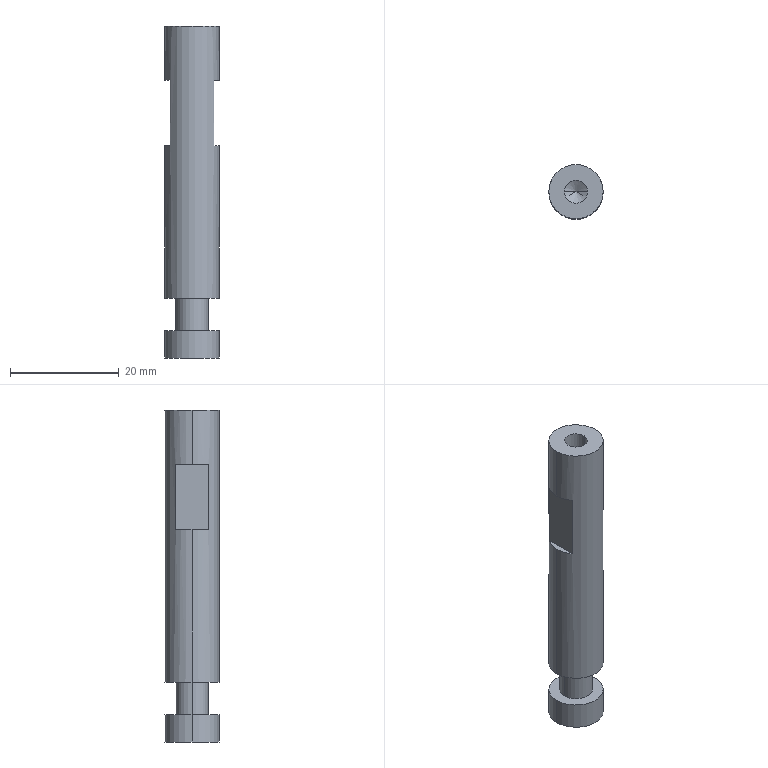Part | STEP file | 2101 Cylinder joint B | 1 solid | 20 faces | box 10 x 10 x 61 mm | volume 4191 mm3 | plane 10 | cylinder 8 | cone 2 | commonest cylinder face diameters 10 x4 4.2 x2 6 x2
STEP:
#1=CARTESIAN_POINT('',(0.,0.,0.));
#2=DIRECTION('',(0.,0.,1.));
#3=DIRECTION('',(1.,0.,0.));
#4=AXIS2_PLACEMENT_3D('',#1,#2,#3);
#5=CARTESIAN_POINT('',(2.1,0.,47.));
#6=VERTEX_POINT('',#5);
#7=CARTESIAN_POINT('',(2.1,0.,61.));
#8=VERTEX_POINT('',#7);
#9=CARTESIAN_POINT('',(2.1,0.,61.));
#10=DIRECTION('',(0.,0.,1.));
#11=VECTOR('',#10,1.);
#12=LINE('',#9,#11);
#13=CARTESIAN_POINT('',(0.,0.,61.));
#14=DIRECTION('',(0.,0.,1.));
#15=DIRECTION('',(1.,0.,0.));
#16=AXIS2_PLACEMENT_3D('',#13,#14,#15);
#17=CYLINDRICAL_SURFACE('',#16,2.1);
#18=CARTESIAN_POINT('',(6.283,0.));
#19=DIRECTION('',(0.,1.));
#20=VECTOR('',#19,1.);
#21=LINE('',#18,#20);
#22=(GEOMETRIC_REPRESENTATION_CONTEXT(2)PARAMETRIC_REPRESENTATION_CONTEXT()REPRESENTATION_CONTEXT('',''));
#23=DEFINITIONAL_REPRESENTATION('',(#21),#22);
#24=PCURVE('',#17,#23);
#25=CARTESIAN_POINT('',(0.,0.,61.));
#26=DIRECTION('',(0.,0.,1.));
#27=DIRECTION('',(1.,0.,0.));
#28=AXIS2_PLACEMENT_3D('',#25,#26,#27);
#29=CYLINDRICAL_SURFACE('',#28,2.1);
#30=CARTESIAN_POINT('',(0.,0.));
#31=DIRECTION('',(0.,1.));
#32=VECTOR('',#31,1.);
#33=LINE('',#30,#32);
#34=(GEOMETRIC_REPRESENTATION_CONTEXT(2)PARAMETRIC_REPRESENTATION_CONTEXT()REPRESENTATION_CONTEXT('',''));
#35=DEFINITIONAL_REPRESENTATION('',(#33),#34);
#36=PCURVE('',#29,#35);
#37=SURFACE_CURVE('',#12,(#24,#36),.PCURVE_S1.);
#38=EDGE_CURVE('',#6,#8,#37,.T.);
#39=ORIENTED_EDGE('',*,*,#38,.T.);
#40=CARTESIAN_POINT('',(-2.1,0.,61.));
#41=VERTEX_POINT('',#40);
#42=CARTESIAN_POINT('',(0.,0.,61.));
#43=DIRECTION('',(0.,0.,1.));
#44=DIRECTION('',(1.,0.,0.));
#45=AXIS2_PLACEMENT_3D('',#42,#43,#44);
#46=CIRCLE('',#45,2.1);
#47=CARTESIAN_POINT('',(0.,0.));
#48=DIRECTION('',(1.,0.));
#49=VECTOR('',#48,1.);
#50=LINE('',#47,#49);
#51=(GEOMETRIC_REPRESENTATION_CONTEXT(2)PARAMETRIC_REPRESENTATION_CONTEXT()REPRESENTATION_CONTEXT('',''));
#52=DEFINITIONAL_REPRESENTATION('',(#50),#51);
#53=PCURVE('',#17,#52);
#54=CARTESIAN_POINT('',(0.,0.,61.));
#55=DIRECTION('',(0.,0.,1.));
#56=DIRECTION('',(1.,0.,0.));
#57=AXIS2_PLACEMENT_3D('',#54,#55,#56);
#58=PLANE('',#57);
#59=CARTESIAN_POINT('',(0.,0.));
#60=DIRECTION('',(1.,0.));
#61=AXIS2_PLACEMENT_2D('',#59,#60);
#62=CIRCLE('',#61,2.1);
#63=(GEOMETRIC_REPRESENTATION_CONTEXT(2)PARAMETRIC_REPRESENTATION_CONTEXT()REPRESENTATION_CONTEXT('',''));
#64=DEFINITIONAL_REPRESENTATION('',(#62),#63);
#65=PCURVE('',#58,#64);
#66=SURFACE_CURVE('',#46,(#53,#65),.PCURVE_S1.);
#67=EDGE_CURVE('',#41,#8,#66,.T.);
#68=ORIENTED_EDGE('',*,*,#67,.F.);
#69=CARTESIAN_POINT('',(-2.1,0.,47.));
#70=VERTEX_POINT('',#69);
#71=CARTESIAN_POINT('',(-2.1,0.,61.));
#72=DIRECTION('',(0.,0.,1.));
#73=VECTOR('',#72,1.);
#74=LINE('',#71,#73);
#75=CARTESIAN_POINT('',(3.142,0.));
#76=DIRECTION('',(0.,1.));
#77=VECTOR('',#76,1.);
#78=LINE('',#75,#77);
#79=(GEOMETRIC_REPRESENTATION_CONTEXT(2)PARAMETRIC_REPRESENTATION_CONTEXT()REPRESENTATION_CONTEXT('',''));
#80=DEFINITIONAL_REPRESENTATION('',(#78),#79);
#81=PCURVE('',#17,#80);
#82=CARTESIAN_POINT('',(3.142,0.));
#83=DIRECTION('',(0.,1.));
#84=VECTOR('',#83,1.);
#85=LINE('',#82,#84);
#86=(GEOMETRIC_REPRESENTATION_CONTEXT(2)PARAMETRIC_REPRESENTATION_CONTEXT()REPRESENTATION_CONTEXT('',''));
#87=DEFINITIONAL_REPRESENTATION('',(#85),#86);
#88=PCURVE('',#29,#87);
#89=SURFACE_CURVE('',#74,(#81,#88),.PCURVE_S1.);
#90=EDGE_CURVE('',#70,#41,#89,.T.);
#91=ORIENTED_EDGE('',*,*,#90,.F.);
#92=CARTESIAN_POINT('',(0.,0.,47.));
#93=DIRECTION('',(0.,0.,1.));
#94=DIRECTION('',(1.,0.,0.));
#95=AXIS2_PLACEMENT_3D('',#92,#93,#94);
#96=CIRCLE('',#95,2.1);
#97=CARTESIAN_POINT('',(0.,-14.));
#98=DIRECTION('',(1.,0.));
#99=VECTOR('',#98,1.);
#100=LINE('',#97,#99);
#101=(GEOMETRIC_REPRESENTATION_CONTEXT(2)PARAMETRIC_REPRESENTATION_CONTEXT()REPRESENTATION_CONTEXT('',''));
#102=DEFINITIONAL_REPRESENTATION('',(#100),#101);
#103=PCURVE('',#17,#102);
#104=CARTESIAN_POINT('',(0.,0.,47.));
#105=DIRECTION('',(0.,0.,1.));
#106=DIRECTION('',(1.,0.,0.));
#107=AXIS2_PLACEMENT_3D('',#104,#105,#106);
#108=CONICAL_SURFACE('',#107,2.1,1.03);
#109=CARTESIAN_POINT('',(0.,0.));
#110=DIRECTION('',(1.,0.));
#111=VECTOR('',#110,1.);
#112=LINE('',#109,#111);
#113=(GEOMETRIC_REPRESENTATION_CONTEXT(2)PARAMETRIC_REPRESENTATION_CONTEXT()REPRESENTATION_CONTEXT('',''));
#114=DEFINITIONAL_REPRESENTATION('',(#112),#113);
#115=PCURVE('',#108,#114);
#116=SURFACE_CURVE('',#96,(#103,#115),.PCURVE_S1.);
#117=EDGE_CURVE('',#70,#6,#116,.T.);
#118=ORIENTED_EDGE('',*,*,#117,.T.);
#119=EDGE_LOOP('',(#39,#68,#91,#118));
#120=FACE_BOUND('',#119,.F.);
#121=ADVANCED_FACE('',(#120),#17,.F.);
#122=ORIENTED_EDGE('',*,*,#117,.F.);
#123=CARTESIAN_POINT('',(0.,0.,45.738));
#124=VERTEX_POINT('',#123);
#125=CARTESIAN_POINT('',(-2.1,0.,47.));
#126=DIRECTION('',(-0.8572,0.,0.515));
#127=VECTOR('',#126,1.);
#128=LINE('',#125,#127);
#129=CARTESIAN_POINT('',(3.142,0.));
#130=DIRECTION('',(0.,1.));
#131=VECTOR('',#130,1.);
#132=LINE('',#129,#131);
#133=(GEOMETRIC_REPRESENTATION_CONTEXT(2)PARAMETRIC_REPRESENTATION_CONTEXT()REPRESENTATION_CONTEXT('',''));
#134=DEFINITIONAL_REPRESENTATION('',(#132),#133);
#135=PCURVE('',#108,#134);
#136=CARTESIAN_POINT('',(0.,0.,47.));
#137=DIRECTION('',(0.,0.,1.));
#138=DIRECTION('',(1.,0.,0.));
#139=AXIS2_PLACEMENT_3D('',#136,#137,#138);
#140=CONICAL_SURFACE('',#139,2.1,1.03);
#141=CARTESIAN_POINT('',(3.142,0.));
#142=DIRECTION('',(0.,1.));
#143=VECTOR('',#142,1.);
#144=LINE('',#141,#143);
#145=(GEOMETRIC_REPRESENTATION_CONTEXT(2)PARAMETRIC_REPRESENTATION_CONTEXT()REPRESENTATION_CONTEXT('',''));
#146=DEFINITIONAL_REPRESENTATION('',(#144),#145);
#147=PCURVE('',#140,#146);
#148=SURFACE_CURVE('',#128,(#135,#147),.PCURVE_S1.);
#149=EDGE_CURVE('',#124,#70,#148,.T.);
#150=ORIENTED_EDGE('',*,*,#149,.F.);
#151=CARTESIAN_POINT('',(2.1,0.,47.));
#152=DIRECTION('',(0.8572,0.,0.515));
#153=VECTOR('',#152,1.);
#154=LINE('',#151,#153);
#155=CARTESIAN_POINT('',(6.283,0.));
#156=DIRECTION('',(0.,1.));
#157=VECTOR('',#156,1.);
#158=LINE('',#155,#157);
#159=(GEOMETRIC_REPRESENTATION_CONTEXT(2)PARAMETRIC_REPRESENTATION_CONTEXT()REPRESENTATION_CONTEXT('',''));
#160=DEFINITIONAL_REPRESENTATION('',(#158),#159);
#161=PCURVE('',#108,#160);
#162=CARTESIAN_POINT('',(0.,0.));
#163=DIRECTION('',(0.,1.));
#164=VECTOR('',#163,1.);
#165=LINE('',#162,#164);
#166=(GEOMETRIC_REPRESENTATION_CONTEXT(2)PARAMETRIC_REPRESENTATION_CONTEXT()REPRESENTATION_CONTEXT('',''));
#167=DEFINITIONAL_REPRESENTATION('',(#165),#166);
#168=PCURVE('',#140,#167);
#169=SURFACE_CURVE('',#154,(#161,#168),.PCURVE_S1.);
#170=EDGE_CURVE('',#124,#6,#169,.T.);
#171=ORIENTED_EDGE('',*,*,#170,.T.);
#172=EDGE_LOOP('',(#122,#150,#171));
#173=FACE_BOUND('',#172,.F.);
#174=ADVANCED_FACE('',(#173),#108,.F.);
#175=CARTESIAN_POINT('',(3.,0.,11.));
#176=VERTEX_POINT('',#175);
#177=CARTESIAN_POINT('',(-3.,0.,11.));
#178=VERTEX_POINT('',#177);
#179=CARTESIAN_POINT('',(0.,0.,11.));
#180=DIRECTION('',(0.,0.,1.));
#181=DIRECTION('',(1.,0.,0.));
#182=AXIS2_PLACEMENT_3D('',#179,#180,#181);
#183=CIRCLE('',#182,3.);
#184=CARTESIAN_POINT('',(0.,0.,11.));
#185=DIRECTION('',(0.,0.,-1.));
#186=DIRECTION('',(-1.,0.,0.));
#187=AXIS2_PLACEMENT_3D('',#184,#185,#186);
#188=CYLINDRICAL_SURFACE('',#187,3.);
#189=CARTESIAN_POINT('',(3.142,0.));
#190=DIRECTION('',(-1.,0.));
#191=VECTOR('',#190,1.);
#192=LINE('',#189,#191);
#193=(GEOMETRIC_REPRESENTATION_CONTEXT(2)PARAMETRIC_REPRESENTATION_CONTEXT()REPRESENTATION_CONTEXT('',''));
#194=DEFINITIONAL_REPRESENTATION('',(#192),#193);
#195=PCURVE('',#188,#194);
#196=CARTESIAN_POINT('',(0.,0.,11.));
#197=DIRECTION('',(0.,0.,1.));
#198=DIRECTION('',(1.,0.,0.));
#199=AXIS2_PLACEMENT_3D('',#196,#197,#198);
#200=PLANE('',#199);
#201=CARTESIAN_POINT('',(0.,0.));
#202=DIRECTION('',(1.,0.));
#203=AXIS2_PLACEMENT_2D('',#201,#202);
#204=CIRCLE('',#203,3.);
#205=(GEOMETRIC_REPRESENTATION_CONTEXT(2)PARAMETRIC_REPRESENTATION_CONTEXT()REPRESENTATION_CONTEXT('',''));
#206=DEFINITIONAL_REPRESENTATION('',(#204),#205);
#207=PCURVE('',#200,#206);
#208=SURFACE_CURVE('',#183,(#195,#207),.PCURVE_S1.);
#209=EDGE_CURVE('',#176,#178,#208,.T.);
#210=ORIENTED_EDGE('',*,*,#209,.F.);
#211=CARTESIAN_POINT('',(3.,0.,5.));
#212=VERTEX_POINT('',#211);
#213=CARTESIAN_POINT('',(3.,0.,11.));
#214=DIRECTION('',(0.,0.,-1.));
#215=VECTOR('',#214,1.);
#216=LINE('',#213,#215);
#217=CARTESIAN_POINT('',(3.142,0.));
#218=DIRECTION('',(0.,1.));
#219=VECTOR('',#218,1.);
#220=LINE('',#217,#219);
#221=(GEOMETRIC_REPRESENTATION_CONTEXT(2)PARAMETRIC_REPRESENTATION_CONTEXT()REPRESENTATION_CONTEXT('',''));
#222=DEFINITIONAL_REPRESENTATION('',(#220),#221);
#223=PCURVE('',#188,#222);
#224=CARTESIAN_POINT('',(0.,0.,11.));
#225=DIRECTION('',(0.,0.,-1.));
#226=DIRECTION('',(-1.,0.,0.));
#227=AXIS2_PLACEMENT_3D('',#224,#225,#226);
#228=CYLINDRICAL_SURFACE('',#227,3.);
#229=CARTESIAN_POINT('',(3.142,0.));
#230=DIRECTION('',(0.,1.));
#231=VECTOR('',#230,1.);
#232=LINE('',#229,#231);
#233=(GEOMETRIC_REPRESENTATION_CONTEXT(2)PARAMETRIC_REPRESENTATION_CONTEXT()REPRESENTATION_CONTEXT('',''));
#234=DEFINITIONAL_REPRESENTATION('',(#232),#233);
#235=PCURVE('',#228,#234);
#236=SURFACE_CURVE('',#216,(#223,#235),.PCURVE_S1.);
#237=EDGE_CURVE('',#176,#212,#236,.T.);
#238=ORIENTED_EDGE('',*,*,#237,.T.);
#239=CARTESIAN_POINT('',(-3.,0.,5.));
#240=VERTEX_POINT('',#239);
#241=CARTESIAN_POINT('',(0.,0.,5.));
#242=DIRECTION('',(0.,0.,1.));
#243=DIRECTION('',(1.,0.,0.));
#244=AXIS2_PLACEMENT_3D('',#241,#242,#243);
#245=CIRCLE('',#244,3.);
#246=CARTESIAN_POINT('',(3.142,6.));
#247=DIRECTION('',(-1.,0.));
#248=VECTOR('',#247,1.);
#249=LINE('',#246,#248);
#250=(GEOMETRIC_REPRESENTATION_CONTEXT(2)PARAMETRIC_REPRESENTATION_CONTEXT()REPRESENTATION_CONTEXT('',''));
#251=DEFINITIONAL_REPRESENTATION('',(#249),#250);
#252=PCURVE('',#188,#251);
#253=CARTESIAN_POINT('',(0.,0.,5.));
#254=DIRECTION('',(0.,0.,1.));
#255=DIRECTION('',(1.,0.,0.));
#256=AXIS2_PLACEMENT_3D('',#253,#254,#255);
#257=PLANE('',#256);
#258=CARTESIAN_POINT('',(0.,0.));
#259=DIRECTION('',(1.,0.));
#260=AXIS2_PLACEMENT_2D('',#258,#259);
#261=CIRCLE('',#260,3.);
#262=(GEOMETRIC_REPRESENTATION_CONTEXT(2)PARAMETRIC_REPRESENTATION_CONTEXT()REPRESENTATION_CONTEXT('',''));
#263=DEFINITIONAL_REPRESENTATION('',(#261),#262);
#264=PCURVE('',#257,#263);
#265=SURFACE_CURVE('',#245,(#252,#264),.PCURVE_S1.);
#266=EDGE_CURVE('',#212,#240,#265,.T.);
#267=ORIENTED_EDGE('',*,*,#266,.T.);
#268=CARTESIAN_POINT('',(-3.,0.,11.));
#269=DIRECTION('',(0.,0.,-1.));
#270=VECTOR('',#269,1.);
#271=LINE('',#268,#270);
#272=CARTESIAN_POINT('',(0.,0.));
#273=DIRECTION('',(0.,1.));
#274=VECTOR('',#273,1.);
#275=LINE('',#272,#274);
#276=(GEOMETRIC_REPRESENTATION_CONTEXT(2)PARAMETRIC_REPRESENTATION_CONTEXT()REPRESENTATION_CONTEXT('',''));
#277=DEFINITIONAL_REPRESENTATION('',(#275),#276);
#278=PCURVE('',#188,#277);
#279=CARTESIAN_POINT('',(6.283,0.));
#280=DIRECTION('',(0.,1.));
#281=VECTOR('',#280,1.);
#282=LINE('',#279,#281);
#283=(GEOMETRIC_REPRESENTATION_CONTEXT(2)PARAMETRIC_REPRESENTATION_CONTEXT()REPRESENTATION_CONTEXT('',''));
#284=DEFINITIONAL_REPRESENTATION('',(#282),#283);
#285=PCURVE('',#228,#284);
#286=SURFACE_CURVE('',#271,(#278,#285),.PCURVE_S1.);
#287=EDGE_CURVE('',#178,#240,#286,.T.);
#288=ORIENTED_EDGE('',*,*,#287,.F.);
#289=EDGE_LOOP('',(#210,#238,#267,#288));
#290=FACE_BOUND('',#289,.T.);
#291=ADVANCED_FACE('',(#290),#188,.T.);
#292=CARTESIAN_POINT('',(5.,0.,5.));
#293=VERTEX_POINT('',#292);
#294=CARTESIAN_POINT('',(-5.,0.,5.));
#295=VERTEX_POINT('',#294);
#296=CARTESIAN_POINT('',(0.,0.,5.));
#297=DIRECTION('',(0.,0.,1.));
#298=DIRECTION('',(1.,0.,0.));
#299=AXIS2_PLACEMENT_3D('',#296,#297,#298);
#300=CIRCLE('',#299,5.);
#301=CARTESIAN_POINT('',(0.,0.,5.));
#302=DIRECTION('',(0.,0.,-1.));
#303=DIRECTION('',(-1.,0.,0.));
#304=AXIS2_PLACEMENT_3D('',#301,#302,#303);
#305=CYLINDRICAL_SURFACE('',#304,5.);
#306=CARTESIAN_POINT('',(3.142,0.));
#307=DIRECTION('',(-1.,0.));
#308=VECTOR('',#307,1.);
#309=LINE('',#306,#308);
#310=(GEOMETRIC_REPRESENTATION_CONTEXT(2)PARAMETRIC_REPRESENTATION_CONTEXT()REPRESENTATION_CONTEXT('',''));
#311=DEFINITIONAL_REPRESENTATION('',(#309),#310);
#312=PCURVE('',#305,#311);
#313=CARTESIAN_POINT('',(0.,0.));
#314=DIRECTION('',(1.,0.));
#315=AXIS2_PLACEMENT_2D('',#313,#314);
#316=CIRCLE('',#315,5.);
#317=(GEOMETRIC_REPRESENTATION_CONTEXT(2)PARAMETRIC_REPRESENTATION_CONTEXT()REPRESENTATION_CONTEXT('',''));
#318=DEFINITIONAL_REPRESENTATION('',(#316),#317);
#319=PCURVE('',#257,#318);
#320=SURFACE_CURVE('',#300,(#312,#319),.PCURVE_S1.);
#321=EDGE_CURVE('',#293,#295,#320,.T.);
#322=ORIENTED_EDGE('',*,*,#321,.F.);
#323=CARTESIAN_POINT('',(5.,0.,0.));
#324=VERTEX_POINT('',#323);
#325=CARTESIAN_POINT('',(5.,0.,5.));
#326=DIRECTION('',(0.,0.,-1.));
#327=VECTOR('',#326,1.);
#328=LINE('',#325,#327);
#329=CARTESIAN_POINT('',(3.142,0.));
#330=DIRECTION('',(0.,1.));
#331=VECTOR('',#330,1.);
#332=LINE('',#329,#331);
#333=(GEOMETRIC_REPRESENTATION_CONTEXT(2)PARAMETRIC_REPRESENTATION_CONTEXT()REPRESENTATION_CONTEXT('',''));
#334=DEFINITIONAL_REPRESENTATION('',(#332),#333);
#335=PCURVE('',#305,#334);
#336=CARTESIAN_POINT('',(0.,0.,5.));
#337=DIRECTION('',(0.,0.,-1.));
#338=DIRECTION('',(-1.,0.,0.));
#339=AXIS2_PLACEMENT_3D('',#336,#337,#338);
#340=CYLINDRICAL_SURFACE('',#339,5.);
#341=CARTESIAN_POINT('',(3.142,0.));
#342=DIRECTION('',(0.,1.));
#343=VECTOR('',#342,1.);
#344=LINE('',#341,#343);
#345=(GEOMETRIC_REPRESENTATION_CONTEXT(2)PARAMETRIC_REPRESENTATION_CONTEXT()REPRESENTATION_CONTEXT('',''));
#346=DEFINITIONAL_REPRESENTATION('',(#344),#345);
#347=PCURVE('',#340,#346);
#348=SURFACE_CURVE('',#328,(#335,#347),.PCURVE_S1.);
#349=EDGE_CURVE('',#293,#324,#348,.T.);
#350=ORIENTED_EDGE('',*,*,#349,.T.);
#351=CARTESIAN_POINT('',(-5.,0.,0.));
#352=VERTEX_POINT('',#351);
#353=CARTESIAN_POINT('',(0.,0.,0.));
#354=DIRECTION('',(0.,0.,1.));
#355=DIRECTION('',(1.,0.,0.));
#356=AXIS2_PLACEMENT_3D('',#353,#354,#355);
#357=CIRCLE('',#356,5.);
#358=CARTESIAN_POINT('',(3.142,5.));
#359=DIRECTION('',(-1.,0.));
#360=VECTOR('',#359,1.);
#361=LINE('',#358,#360);
#362=(GEOMETRIC_REPRESENTATION_CONTEXT(2)PARAMETRIC_REPRESENTATION_CONTEXT()REPRESENTATION_CONTEXT('',''));
#363=DEFINITIONAL_REPRESENTATION('',(#361),#362);
#364=PCURVE('',#305,#363);
#365=CARTESIAN_POINT('',(0.,0.,0.));
#366=DIRECTION('',(0.,0.,1.));
#367=DIRECTION('',(1.,0.,0.));
#368=AXIS2_PLACEMENT_3D('',#365,#366,#367);
#369=PLANE('',#368);
#370=CARTESIAN_POINT('',(0.,0.));
#371=DIRECTION('',(1.,0.));
#372=AXIS2_PLACEMENT_2D('',#370,#371);
#373=CIRCLE('',#372,5.);
#374=(GEOMETRIC_REPRESENTATION_CONTEXT(2)PARAMETRIC_REPRESENTATION_CONTEXT()REPRESENTATION_CONTEXT('',''));
#375=DEFINITIONAL_REPRESENTATION('',(#373),#374);
#376=PCURVE('',#369,#375);
#377=SURFACE_CURVE('',#357,(#364,#376),.PCURVE_S1.);
#378=EDGE_CURVE('',#324,#352,#377,.T.);
#379=ORIENTED_EDGE('',*,*,#378,.T.);
#380=CARTESIAN_POINT('',(-5.,0.,5.));
#381=DIRECTION('',(0.,0.,-1.));
#382=VECTOR('',#381,1.);
#383=LINE('',#380,#382);
#384=CARTESIAN_POINT('',(0.,0.));
#385=DIRECTION('',(0.,1.));
#386=VECTOR('',#385,1.);
#387=LINE('',#384,#386);
#388=(GEOMETRIC_REPRESENTATION_CONTEXT(2)PARAMETRIC_REPRESENTATION_CONTEXT()REPRESENTATION_CONTEXT('',''));
#389=DEFINITIONAL_REPRESENTATION('',(#387),#388);
#390=PCURVE('',#305,#389);
#391=CARTESIAN_POINT('',(6.283,0.));
#392=DIRECTION('',(0.,1.));
#393=VECTOR('',#392,1.);
#394=LINE('',#391,#393);
#395=(GEOMETRIC_REPRESENTATION_CONTEXT(2)PARAMETRIC_REPRESENTATION_CONTEXT()REPRESENTATION_CONTEXT('',''));
#396=DEFINITIONAL_REPRESENTATION('',(#394),#395);
#397=PCURVE('',#340,#396);
#398=SURFACE_CURVE('',#383,(#390,#397),.PCURVE_S1.);
#399=EDGE_CURVE('',#295,#352,#398,.T.);
#400=ORIENTED_EDGE('',*,*,#399,.F.);
#401=EDGE_LOOP('',(#322,#350,#379,#400));
#402=FACE_BOUND('',#401,.T.);
#403=ADVANCED_FACE('',(#402),#305,.T.);
#404=CARTESIAN_POINT('',(5.,0.,61.));
#405=VERTEX_POINT('',#404);
#406=CARTESIAN_POINT('',(-5.,0.,61.));
#407=VERTEX_POINT('',#406);
#408=CARTESIAN_POINT('',(0.,0.,61.));
#409=DIRECTION('',(0.,0.,1.));
#410=DIRECTION('',(1.,0.,0.));
#411=AXIS2_PLACEMENT_3D('',#408,#409,#410);
#412=CIRCLE('',#411,5.);
#413=CARTESIAN_POINT('',(0.,0.,61.));
#414=DIRECTION('',(0.,0.,-1.));
#415=DIRECTION('',(-1.,0.,0.));
#416=AXIS2_PLACEMENT_3D('',#413,#414,#415);
#417=CYLINDRICAL_SURFACE('',#416,5.);
#418=CARTESIAN_POINT('',(3.142,0.));
#419=DIRECTION('',(-1.,0.));
#420=VECTOR('',#419,1.);
#421=LINE('',#418,#420);
#422=(GEOMETRIC_REPRESENTATION_CONTEXT(2)PARAMETRIC_REPRESENTATION_CONTEXT()REPRESENTATION_CONTEXT('',''));
#423=DEFINITIONAL_REPRESENTATION('',(#421),#422);
#424=PCURVE('',#417,#423);
#425=CARTESIAN_POINT('',(0.,0.));
#426=DIRECTION('',(1.,0.));
#427=AXIS2_PLACEMENT_2D('',#425,#426);
#428=CIRCLE('',#427,5.);
#429=(GEOMETRIC_REPRESENTATION_CONTEXT(2)PARAMETRIC_REPRESENTATION_CONTEXT()REPRESENTATION_CONTEXT('',''));
#430=DEFINITIONAL_REPRESENTATION('',(#428),#429);
#431=PCURVE('',#58,#430);
#432=SURFACE_CURVE('',#412,(#424,#431),.PCURVE_S1.);
#433=EDGE_CURVE('',#405,#407,#432,.T.);
#434=ORIENTED_EDGE('',*,*,#433,.F.);
#435=CARTESIAN_POINT('',(5.,0.,51.));
#436=VERTEX_POINT('',#435);
#437=CARTESIAN_POINT('',(5.,0.,61.));
#438=DIRECTION('',(0.,0.,-1.));
#439=VECTOR('',#438,1.);
#440=LINE('',#437,#439);
#441=CARTESIAN_POINT('',(3.142,0.));
#442=DIRECTION('',(0.,1.));
#443=VECTOR('',#442,1.);
#444=LINE('',#441,#443);
#445=(GEOMETRIC_REPRESENTATION_CONTEXT(2)PARAMETRIC_REPRESENTATION_CONTEXT()REPRESENTATION_CONTEXT('',''));
#446=DEFINITIONAL_REPRESENTATION('',(#444),#445);
#447=PCURVE('',#417,#446);
#448=CARTESIAN_POINT('',(0.,0.,61.));
#449=DIRECTION('',(0.,0.,-1.));
#450=DIRECTION('',(-1.,0.,0.));
#451=AXIS2_PLACEMENT_3D('',#448,#449,#450);
#452=CYLINDRICAL_SURFACE('',#451,5.);
#453=CARTESIAN_POINT('',(3.142,0.));
#454=DIRECTION('',(0.,1.));
#455=VECTOR('',#454,1.);
#456=LINE('',#453,#455);
#457=(GEOMETRIC_REPRESENTATION_CONTEXT(2)PARAMETRIC_REPRESENTATION_CONTEXT()REPRESENTATION_CONTEXT('',''));
#458=DEFINITIONAL_REPRESENTATION('',(#456),#457);
#459=PCURVE('',#452,#458);
#460=SURFACE_CURVE('',#440,(#447,#459),.PCURVE_S1.);
#461=EDGE_CURVE('',#405,#436,#460,.T.);
#462=ORIENTED_EDGE('',*,*,#461,.T.);
#463=CARTESIAN_POINT('',(4.,3.,51.));
#464=VERTEX_POINT('',#463);
#465=CARTESIAN_POINT('',(0.,0.,51.));
#466=DIRECTION('',(0.,0.,-1.));
#467=DIRECTION('',(-1.,0.,0.));
#468=AXIS2_PLACEMENT_3D('',#465,#466,#467);
#469=CIRCLE('',#468,5.);
#470=CARTESIAN_POINT('',(0.,10.));
#471=DIRECTION('',(1.,0.));
#472=VECTOR('',#471,1.);
#473=LINE('',#470,#472);
#474=(GEOMETRIC_REPRESENTATION_CONTEXT(2)PARAMETRIC_REPRESENTATION_CONTEXT()REPRESENTATION_CONTEXT('',''));
#475=DEFINITIONAL_REPRESENTATION('',(#473),#474);
#476=PCURVE('',#417,#475);
#477=CARTESIAN_POINT('',(11.893,50.,51.));
#478=DIRECTION('',(0.,0.,-1.));
#479=DIRECTION('',(-1.,0.,0.));
#480=AXIS2_PLACEMENT_3D('',#477,#478,#479);
#481=PLANE('',#480);
#482=CARTESIAN_POINT('',(11.893,-50.));
#483=DIRECTION('',(1.,0.));
#484=AXIS2_PLACEMENT_2D('',#482,#483);
#485=CIRCLE('',#484,5.);
#486=(GEOMETRIC_REPRESENTATION_CONTEXT(2)PARAMETRIC_REPRESENTATION_CONTEXT()REPRESENTATION_CONTEXT('',''));
#487=DEFINITIONAL_REPRESENTATION('',(#485),#486);
#488=PCURVE('',#481,#487);
#489=SURFACE_CURVE('',#469,(#476,#488),.PCURVE_S1.);
#490=EDGE_CURVE('',#464,#436,#489,.T.);
#491=ORIENTED_EDGE('',*,*,#490,.F.);
#492=CARTESIAN_POINT('',(4.,3.,39.));
#493=VERTEX_POINT('',#492);
#494=CARTESIAN_POINT('',(4.,3.,61.));
#495=DIRECTION('',(0.,0.,1.));
#496=VECTOR('',#495,1.);
#497=LINE('',#494,#496);
#498=CARTESIAN_POINT('',(2.498,0.));
#499=DIRECTION('',(0.,-1.));
#500=VECTOR('',#499,1.);
#501=LINE('',#498,#500);
#502=(GEOMETRIC_REPRESENTATION_CONTEXT(2)PARAMETRIC_REPRESENTATION_CONTEXT()REPRESENTATION_CONTEXT('',''));
#503=DEFINITIONAL_REPRESENTATION('',(#501),#502);
#504=PCURVE('',#417,#503);
#505=CARTESIAN_POINT('',(4.,50.,39.));
#506=DIRECTION('',(1.,0.,0.));
#507=DIRECTION('',(0.,0.,-1.));
#508=AXIS2_PLACEMENT_3D('',#505,#506,#507);
#509=PLANE('',#508);
#510=CARTESIAN_POINT('',(-22.,-47.));
#511=DIRECTION('',(-1.,0.));
#512=VECTOR('',#511,1.);
#513=LINE('',#510,#512);
#514=(GEOMETRIC_REPRESENTATION_CONTEXT(2)PARAMETRIC_REPRESENTATION_CONTEXT()REPRESENTATION_CONTEXT('',''));
#515=DEFINITIONAL_REPRESENTATION('',(#513),#514);
#516=PCURVE('',#509,#515);
#517=SURFACE_CURVE('',#497,(#504,#516),.PCURVE_S1.);
#518=EDGE_CURVE('',#493,#464,#517,.T.);
#519=ORIENTED_EDGE('',*,*,#518,.F.);
#520=CARTESIAN_POINT('',(5.,0.,39.));
#521=VERTEX_POINT('',#520);
#522=CARTESIAN_POINT('',(0.,0.,39.));
#523=DIRECTION('',(0.,0.,1.));
#524=DIRECTION('',(1.,0.,0.));
#525=AXIS2_PLACEMENT_3D('',#522,#523,#524);
#526=CIRCLE('',#525,5.);
#527=CARTESIAN_POINT('',(3.142,22.));
#528=DIRECTION('',(-1.,0.));
#529=VECTOR('',#528,1.);
#530=LINE('',#527,#529);
#531=(GEOMETRIC_REPRESENTATION_CONTEXT(2)PARAMETRIC_REPRESENTATION_CONTEXT()REPRESENTATION_CONTEXT('',''));
#532=DEFINITIONAL_REPRESENTATION('',(#530),#531);
#533=PCURVE('',#417,#532);
#534=CARTESIAN_POINT('',(11.893,50.,39.));
#535=DIRECTION('',(0.,0.,1.));
#536=DIRECTION('',(1.,0.,0.));
#537=AXIS2_PLACEMENT_3D('',#534,#535,#536);
#538=PLANE('',#537);
#539=CARTESIAN_POINT('',(-11.893,-50.));
#540=DIRECTION('',(1.,0.));
#541=AXIS2_PLACEMENT_2D('',#539,#540);
#542=CIRCLE('',#541,5.);
#543=(GEOMETRIC_REPRESENTATION_CONTEXT(2)PARAMETRIC_REPRESENTATION_CONTEXT()REPRESENTATION_CONTEXT('',''));
#544=DEFINITIONAL_REPRESENTATION('',(#542),#543);
#545=PCURVE('',#538,#544);
#546=SURFACE_CURVE('',#526,(#533,#545),.PCURVE_S1.);
#547=EDGE_CURVE('',#521,#493,#546,.T.);
#548=ORIENTED_EDGE('',*,*,#547,.F.);
#549=CARTESIAN_POINT('',(5.,0.,11.));
#550=VERTEX_POINT('',#549);
#551=CARTESIAN_POINT('',(5.,0.,61.));
#552=DIRECTION('',(0.,0.,-1.));
#553=VECTOR('',#552,1.);
#554=LINE('',#551,#553);
#555=CARTESIAN_POINT('',(3.142,0.));
#556=DIRECTION('',(0.,1.));
#557=VECTOR('',#556,1.);
#558=LINE('',#555,#557);
#559=(GEOMETRIC_REPRESENTATION_CONTEXT(2)PARAMETRIC_REPRESENTATION_CONTEXT()REPRESENTATION_CONTEXT('',''));
#560=DEFINITIONAL_REPRESENTATION('',(#558),#559);
#561=PCURVE('',#417,#560);
#562=CARTESIAN_POINT('',(3.142,0.));
#563=DIRECTION('',(0.,1.));
#564=VECTOR('',#563,1.);
#565=LINE('',#562,#564);
#566=(GEOMETRIC_REPRESENTATION_CONTEXT(2)PARAMETRIC_REPRESENTATION_CONTEXT()REPRESENTATION_CONTEXT('',''));
#567=DEFINITIONAL_REPRESENTATION('',(#565),#566);
#568=PCURVE('',#452,#567);
#569=SURFACE_CURVE('',#554,(#561,#568),.PCURVE_S1.);
#570=EDGE_CURVE('',#521,#550,#569,.T.);
#571=ORIENTED_EDGE('',*,*,#570,.T.);
#572=CARTESIAN_POINT('',(-5.,0.,11.));
#573=VERTEX_POINT('',#572);
#574=CARTESIAN_POINT('',(0.,0.,11.));
#575=DIRECTION('',(0.,0.,1.));
#576=DIRECTION('',(1.,0.,0.));
#577=AXIS2_PLACEMENT_3D('',#574,#575,#576);
#578=CIRCLE('',#577,5.);
#579=CARTESIAN_POINT('',(3.142,50.));
#580=DIRECTION('',(-1.,0.));
#581=VECTOR('',#580,1.);
#582=LINE('',#579,#581);
#583=(GEOMETRIC_REPRESENTATION_CONTEXT(2)PARAMETRIC_REPRESENTATION_CONTEXT()REPRESENTATION_CONTEXT('',''));
#584=DEFINITIONAL_REPRESENTATION('',(#582),#583);
#585=PCURVE('',#417,#584);
#586=CARTESIAN_POINT('',(0.,0.));
#587=DIRECTION('',(1.,0.));
#588=AXIS2_PLACEMENT_2D('',#586,#587);
#589=CIRCLE('',#588,5.);
#590=(GEOMETRIC_REPRESENTATION_CONTEXT(2)PARAMETRIC_REPRESENTATION_CONTEXT()REPRESENTATION_CONTEXT('',''));
#591=DEFINITIONAL_REPRESENTATION('',(#589),#590);
#592=PCURVE('',#200,#591);
#593=SURFACE_CURVE('',#578,(#585,#592),.PCURVE_S1.);
#594=EDGE_CURVE('',#550,#573,#593,.T.);
#595=ORIENTED_EDGE('',*,*,#594,.T.);
#596=CARTESIAN_POINT('',(-5.,0.,39.));
#597=VERTEX_POINT('',#596);
#598=CARTESIAN_POINT('',(-5.,0.,61.));
#599=DIRECTION('',(0.,0.,-1.));
#600=VECTOR('',#599,1.);
#601=LINE('',#598,#600);
#602=CARTESIAN_POINT('',(0.,0.));
#603=DIRECTION('',(0.,1.));
#604=VECTOR('',#603,1.);
#605=LINE('',#602,#604);
#606=(GEOMETRIC_REPRESENTATION_CONTEXT(2)PARAMETRIC_REPRESENTATION_CONTEXT()REPRESENTATION_CONTEXT('',''));
#607=DEFINITIONAL_REPRESENTATION('',(#605),#606);
#608=PCURVE('',#417,#607);
#609=CARTESIAN_POINT('',(6.283,0.));
#610=DIRECTION('',(0.,1.));
#611=VECTOR('',#610,1.);
#612=LINE('',#609,#611);
#613=(GEOMETRIC_REPRESENTATION_CONTEXT(2)PARAMETRIC_REPRESENTATION_CONTEXT()REPRESENTATION_CONTEXT('',''));
#614=DEFINITIONAL_REPRESENTATION('',(#612),#613);
#615=PCURVE('',#452,#614);
#616=SURFACE_CURVE('',#601,(#608,#615),.PCURVE_S1.);
#617=EDGE_CURVE('',#597,#573,#616,.T.);
#618=ORIENTED_EDGE('',*,*,#617,.F.);
#619=CARTESIAN_POINT('',(-4.,3.,39.));
#620=VERTEX_POINT('',#619);
#621=CARTESIAN_POINT('',(0.,0.,39.));
#622=DIRECTION('',(0.,0.,1.));
#623=DIRECTION('',(1.,0.,0.));
#624=AXIS2_PLACEMENT_3D('',#621,#622,#623);
#625=CIRCLE('',#624,5.);
#626=CARTESIAN_POINT('',(3.142,22.));
#627=DIRECTION('',(-1.,0.));
#628=VECTOR('',#627,1.);
#629=LINE('',#626,#628);
#630=(GEOMETRIC_REPRESENTATION_CONTEXT(2)PARAMETRIC_REPRESENTATION_CONTEXT()REPRESENTATION_CONTEXT('',''));
#631=DEFINITIONAL_REPRESENTATION('',(#629),#630);
#632=PCURVE('',#417,#631);
#633=CARTESIAN_POINT('',(-11.893,50.,39.));
#634=DIRECTION('',(0.,0.,1.));
#635=DIRECTION('',(1.,0.,0.));
#636=AXIS2_PLACEMENT_3D('',#633,#634,#635);
#637=PLANE('',#636);
#638=CARTESIAN_POINT('',(11.893,-50.));
#639=DIRECTION('',(1.,0.));
#640=AXIS2_PLACEMENT_2D('',#638,#639);
#641=CIRCLE('',#640,5.);
#642=(GEOMETRIC_REPRESENTATION_CONTEXT(2)PARAMETRIC_REPRESENTATION_CONTEXT()REPRESENTATION_CONTEXT('',''));
#643=DEFINITIONAL_REPRESENTATION('',(#641),#642);
#644=PCURVE('',#637,#643);
#645=SURFACE_CURVE('',#625,(#632,#644),.PCURVE_S1.);
#646=EDGE_CURVE('',#620,#597,#645,.T.);
#647=ORIENTED_EDGE('',*,*,#646,.F.);
#648=CARTESIAN_POINT('',(-4.,3.,51.));
#649=VERTEX_POINT('',#648);
#650=CARTESIAN_POINT('',(-4.,3.,61.));
#651=DIRECTION('',(0.,0.,-1.));
#652=VECTOR('',#651,1.);
#653=LINE('',#650,#652);
#654=CARTESIAN_POINT('',(0.6435,0.));
#655=DIRECTION('',(0.,1.));
#656=VECTOR('',#655,1.);
#657=LINE('',#654,#656);
#658=(GEOMETRIC_REPRESENTATION_CONTEXT(2)PARAMETRIC_REPRESENTATION_CONTEXT()REPRESENTATION_CONTEXT('',''));
#659=DEFINITIONAL_REPRESENTATION('',(#657),#658);
#660=PCURVE('',#417,#659);
#661=CARTESIAN_POINT('',(-4.,50.,39.));
#662=DIRECTION('',(-1.,0.,0.));
#663=DIRECTION('',(0.,0.,1.));
#664=AXIS2_PLACEMENT_3D('',#661,#662,#663);
#665=PLANE('',#664);
#666=CARTESIAN_POINT('',(22.,-47.));
#667=DIRECTION('',(-1.,0.));
#668=VECTOR('',#667,1.);
#669=LINE('',#666,#668);
#670=(GEOMETRIC_REPRESENTATION_CONTEXT(2)PARAMETRIC_REPRESENTATION_CONTEXT()REPRESENTATION_CONTEXT('',''));
#671=DEFINITIONAL_REPRESENTATION('',(#669),#670);
#672=PCURVE('',#665,#671);
#673=SURFACE_CURVE('',#653,(#660,#672),.PCURVE_S1.);
#674=EDGE_CURVE('',#649,#620,#673,.T.);
#675=ORIENTED_EDGE('',*,*,#674,.F.);
#676=CARTESIAN_POINT('',(-5.,0.,51.));
#677=VERTEX_POINT('',#676);
#678=CARTESIAN_POINT('',(0.,0.,51.));
#679=DIRECTION('',(0.,0.,-1.));
#680=DIRECTION('',(-1.,0.,0.));
#681=AXIS2_PLACEMENT_3D('',#678,#679,#680);
#682=CIRCLE('',#681,5.);
#683=CARTESIAN_POINT('',(0.,10.));
#684=DIRECTION('',(1.,0.));
#685=VECTOR('',#684,1.);
#686=LINE('',#683,#685);
#687=(GEOMETRIC_REPRESENTATION_CONTEXT(2)PARAMETRIC_REPRESENTATION_CONTEXT()REPRESENTATION_CONTEXT('',''));
#688=DEFINITIONAL_REPRESENTATION('',(#686),#687);
#689=PCURVE('',#417,#688);
#690=CARTESIAN_POINT('',(-11.893,50.,51.));
#691=DIRECTION('',(0.,0.,-1.));
#692=DIRECTION('',(-1.,0.,0.));
#693=AXIS2_PLACEMENT_3D('',#690,#691,#692);
#694=PLANE('',#693);
#695=CARTESIAN_POINT('',(-11.893,-50.));
#696=DIRECTION('',(1.,0.));
#697=AXIS2_PLACEMENT_2D('',#695,#696);
#698=CIRCLE('',#697,5.);
#699=(GEOMETRIC_REPRESENTATION_CONTEXT(2)PARAMETRIC_REPRESENTATION_CONTEXT()REPRESENTATION_CONTEXT('',''));
#700=DEFINITIONAL_REPRESENTATION('',(#698),#699);
#701=PCURVE('',#694,#700);
#702=SURFACE_CURVE('',#682,(#689,#701),.PCURVE_S1.);
#703=EDGE_CURVE('',#677,#649,#702,.T.);
#704=ORIENTED_EDGE('',*,*,#703,.F.);
#705=CARTESIAN_POINT('',(-5.,0.,61.));
#706=DIRECTION('',(0.,0.,-1.));
#707=VECTOR('',#706,1.);
#708=LINE('',#705,#707);
#709=CARTESIAN_POINT('',(0.,0.));
#710=DIRECTION('',(0.,1.));
#711=VECTOR('',#710,1.);
#712=LINE('',#709,#711);
#713=(GEOMETRIC_REPRESENTATION_CONTEXT(2)PARAMETRIC_REPRESENTATION_CONTEXT()REPRESENTATION_CONTEXT('',''));
#714=DEFINITIONAL_REPRESENTATION('',(#712),#713);
#715=PCURVE('',#417,#714);
#716=CARTESIAN_POINT('',(6.283,0.));
#717=DIRECTION('',(0.,1.));
#718=VECTOR('',#717,1.);
#719=LINE('',#716,#718);
#720=(GEOMETRIC_REPRESENTATION_CONTEXT(2)PARAMETRIC_REPRESENTATION_CONTEXT()REPRESENTATION_CONTEXT('',''));
#721=DEFINITIONAL_REPRESENTATION('',(#719),#720);
#722=PCURVE('',#452,#721);
#723=SURFACE_CURVE('',#708,(#715,#722),.PCURVE_S1.);
#724=EDGE_CURVE('',#407,#677,#723,.T.);
#725=ORIENTED_EDGE('',*,*,#724,.F.);
#726=EDGE_LOOP('',(#434,#462,#491,#519,#548,#571,#595,#618,#647,#675,#704,#725));
#727=FACE_BOUND('',#726,.T.);
#728=ADVANCED_FACE('',(#727),#417,.T.);
#729=ORIENTED_EDGE('',*,*,#461,.F.);
#730=CARTESIAN_POINT('',(0.,0.,61.));
#731=DIRECTION('',(0.,0.,1.));
#732=DIRECTION('',(1.,0.,0.));
#733=AXIS2_PLACEMENT_3D('',#730,#731,#732);
#734=CIRCLE('',#733,5.);
#735=CARTESIAN_POINT('',(9.425,0.));
#736=DIRECTION('',(-1.,0.));
#737=VECTOR('',#736,1.);
#738=LINE('',#735,#737);
#739=(GEOMETRIC_REPRESENTATION_CONTEXT(2)PARAMETRIC_REPRESENTATION_CONTEXT()REPRESENTATION_CONTEXT('',''));
#740=DEFINITIONAL_REPRESENTATION('',(#738),#739);
#741=PCURVE('',#452,#740);
#742=CARTESIAN_POINT('',(0.,0.));
#743=DIRECTION('',(1.,0.));
#744=AXIS2_PLACEMENT_2D('',#742,#743);
#745=CIRCLE('',#744,5.);
#746=(GEOMETRIC_REPRESENTATION_CONTEXT(2)PARAMETRIC_REPRESENTATION_CONTEXT()REPRESENTATION_CONTEXT('',''));
#747=DEFINITIONAL_REPRESENTATION('',(#745),#746);
#748=PCURVE('',#58,#747);
#749=SURFACE_CURVE('',#734,(#741,#748),.PCURVE_S1.);
#750=EDGE_CURVE('',#407,#405,#749,.T.);
#751=ORIENTED_EDGE('',*,*,#750,.F.);
#752=ORIENTED_EDGE('',*,*,#724,.T.);
#753=CARTESIAN_POINT('',(-4.,-3.,51.));
#754=VERTEX_POINT('',#753);
#755=CARTESIAN_POINT('',(0.,0.,51.));
#756=DIRECTION('',(0.,0.,-1.));
#757=DIRECTION('',(-1.,0.,0.));
#758=AXIS2_PLACEMENT_3D('',#755,#756,#757);
#759=CIRCLE('',#758,5.);
#760=CARTESIAN_POINT('',(0.,10.));
#761=DIRECTION('',(1.,0.));
#762=VECTOR('',#761,1.);
#763=LINE('',#760,#762);
#764=(GEOMETRIC_REPRESENTATION_CONTEXT(2)PARAMETRIC_REPRESENTATION_CONTEXT()REPRESENTATION_CONTEXT('',''));
#765=DEFINITIONAL_REPRESENTATION('',(#763),#764);
#766=PCURVE('',#452,#765);
#767=CARTESIAN_POINT('',(-11.893,-50.));
#768=DIRECTION('',(1.,0.));
#769=AXIS2_PLACEMENT_2D('',#767,#768);
#770=CIRCLE('',#769,5.);
#771=(GEOMETRIC_REPRESENTATION_CONTEXT(2)PARAMETRIC_REPRESENTATION_CONTEXT()REPRESENTATION_CONTEXT('',''));
#772=DEFINITIONAL_REPRESENTATION('',(#770),#771);
#773=PCURVE('',#694,#772);
#774=SURFACE_CURVE('',#759,(#766,#773),.PCURVE_S1.);
#775=EDGE_CURVE('',#754,#677,#774,.T.);
#776=ORIENTED_EDGE('',*,*,#775,.F.);
#777=CARTESIAN_POINT('',(-4.,-3.,39.));
#778=VERTEX_POINT('',#777);
#779=CARTESIAN_POINT('',(-4.,-3.,61.));
#780=DIRECTION('',(0.,0.,1.));
#781=VECTOR('',#780,1.);
#782=LINE('',#779,#781);
#783=CARTESIAN_POINT('',(5.64,0.));
#784=DIRECTION('',(0.,-1.));
#785=VECTOR('',#784,1.);
#786=LINE('',#783,#785);
#787=(GEOMETRIC_REPRESENTATION_CONTEXT(2)PARAMETRIC_REPRESENTATION_CONTEXT()REPRESENTATION_CONTEXT('',''));
#788=DEFINITIONAL_REPRESENTATION('',(#786),#787);
#789=PCURVE('',#452,#788);
#790=CARTESIAN_POINT('',(22.,-53.));
#791=DIRECTION('',(1.,0.));
#792=VECTOR('',#791,1.);
#793=LINE('',#790,#792);
#794=(GEOMETRIC_REPRESENTATION_CONTEXT(2)PARAMETRIC_REPRESENTATION_CONTEXT()REPRESENTATION_CONTEXT('',''));
#795=DEFINITIONAL_REPRESENTATION('',(#793),#794);
#796=PCURVE('',#665,#795);
#797=SURFACE_CURVE('',#782,(#789,#796),.PCURVE_S1.);
#798=EDGE_CURVE('',#778,#754,#797,.T.);
#799=ORIENTED_EDGE('',*,*,#798,.F.);
#800=CARTESIAN_POINT('',(0.,0.,39.));
#801=DIRECTION('',(0.,0.,1.));
#802=DIRECTION('',(1.,0.,0.));
#803=AXIS2_PLACEMENT_3D('',#800,#801,#802);
#804=CIRCLE('',#803,5.);
#805=CARTESIAN_POINT('',(9.425,22.));
#806=DIRECTION('',(-1.,0.));
#807=VECTOR('',#806,1.);
#808=LINE('',#805,#807);
#809=(GEOMETRIC_REPRESENTATION_CONTEXT(2)PARAMETRIC_REPRESENTATION_CONTEXT()REPRESENTATION_CONTEXT('',''));
#810=DEFINITIONAL_REPRESENTATION('',(#808),#809);
#811=PCURVE('',#452,#810);
#812=CARTESIAN_POINT('',(11.893,-50.));
#813=DIRECTION('',(1.,0.));
#814=AXIS2_PLACEMENT_2D('',#812,#813);
#815=CIRCLE('',#814,5.);
#816=(GEOMETRIC_REPRESENTATION_CONTEXT(2)PARAMETRIC_REPRESENTATION_CONTEXT()REPRESENTATION_CONTEXT('',''));
#817=DEFINITIONAL_REPRESENTATION('',(#815),#816);
#818=PCURVE('',#637,#817);
#819=SURFACE_CURVE('',#804,(#811,#818),.PCURVE_S1.);
#820=EDGE_CURVE('',#597,#778,#819,.T.);
#821=ORIENTED_EDGE('',*,*,#820,.F.);
#822=ORIENTED_EDGE('',*,*,#617,.T.);
#823=CARTESIAN_POINT('',(0.,0.,11.));
#824=DIRECTION('',(0.,0.,1.));
#825=DIRECTION('',(1.,0.,0.));
#826=AXIS2_PLACEMENT_3D('',#823,#824,#825);
#827=CIRCLE('',#826,5.);
#828=CARTESIAN_POINT('',(9.425,50.));
#829=DIRECTION('',(-1.,0.));
#830=VECTOR('',#829,1.);
#831=LINE('',#828,#830);
#832=(GEOMETRIC_REPRESENTATION_CONTEXT(2)PARAMETRIC_REPRESENTATION_CONTEXT()REPRESENTATION_CONTEXT('',''));
#833=DEFINITIONAL_REPRESENTATION('',(#831),#832);
#834=PCURVE('',#452,#833);
#835=CARTESIAN_POINT('',(0.,0.));
#836=DIRECTION('',(1.,0.));
#837=AXIS2_PLACEMENT_2D('',#835,#836);
#838=CIRCLE('',#837,5.);
#839=(GEOMETRIC_REPRESENTATION_CONTEXT(2)PARAMETRIC_REPRESENTATION_CONTEXT()REPRESENTATION_CONTEXT('',''));
#840=DEFINITIONAL_REPRESENTATION('',(#838),#839);
#841=PCURVE('',#200,#840);
#842=SURFACE_CURVE('',#827,(#834,#841),.PCURVE_S1.);
#843=EDGE_CURVE('',#573,#550,#842,.T.);
#844=ORIENTED_EDGE('',*,*,#843,.T.);
#845=ORIENTED_EDGE('',*,*,#570,.F.);
#846=CARTESIAN_POINT('',(4.,-3.,39.));
#847=VERTEX_POINT('',#846);
#848=CARTESIAN_POINT('',(0.,0.,39.));
#849=DIRECTION('',(0.,0.,1.));
#850=DIRECTION('',(1.,0.,0.));
#851=AXIS2_PLACEMENT_3D('',#848,#849,#850);
#852=CIRCLE('',#851,5.);
#853=CARTESIAN_POINT('',(9.425,22.));
#854=DIRECTION('',(-1.,0.));
#855=VECTOR('',#854,1.);
#856=LINE('',#853,#855);
#857=(GEOMETRIC_REPRESENTATION_CONTEXT(2)PARAMETRIC_REPRESENTATION_CONTEXT()REPRESENTATION_CONTEXT('',''));
#858=DEFINITIONAL_REPRESENTATION('',(#856),#857);
#859=PCURVE('',#452,#858);
#860=CARTESIAN_POINT('',(-11.893,-50.));
#861=DIRECTION('',(1.,0.));
#862=AXIS2_PLACEMENT_2D('',#860,#861);
#863=CIRCLE('',#862,5.);
#864=(GEOMETRIC_REPRESENTATION_CONTEXT(2)PARAMETRIC_REPRESENTATION_CONTEXT()REPRESENTATION_CONTEXT('',''));
#865=DEFINITIONAL_REPRESENTATION('',(#863),#864);
#866=PCURVE('',#538,#865);
#867=SURFACE_CURVE('',#852,(#859,#866),.PCURVE_S1.);
#868=EDGE_CURVE('',#847,#521,#867,.T.);
#869=ORIENTED_EDGE('',*,*,#868,.F.);
#870=CARTESIAN_POINT('',(4.,-3.,51.));
#871=VERTEX_POINT('',#870);
#872=CARTESIAN_POINT('',(4.,-3.,61.));
#873=DIRECTION('',(0.,0.,-1.));
#874=VECTOR('',#873,1.);
#875=LINE('',#872,#874);
#876=CARTESIAN_POINT('',(3.785,0.));
#877=DIRECTION('',(0.,1.));
#878=VECTOR('',#877,1.);
#879=LINE('',#876,#878);
#880=(GEOMETRIC_REPRESENTATION_CONTEXT(2)PARAMETRIC_REPRESENTATION_CONTEXT()REPRESENTATION_CONTEXT('',''));
#881=DEFINITIONAL_REPRESENTATION('',(#879),#880);
#882=PCURVE('',#452,#881);
#883=CARTESIAN_POINT('',(-22.,-53.));
#884=DIRECTION('',(1.,0.));
#885=VECTOR('',#884,1.);
#886=LINE('',#883,#885);
#887=(GEOMETRIC_REPRESENTATION_CONTEXT(2)PARAMETRIC_REPRESENTATION_CONTEXT()REPRESENTATION_CONTEXT('',''));
#888=DEFINITIONAL_REPRESENTATION('',(#886),#887);
#889=PCURVE('',#509,#888);
#890=SURFACE_CURVE('',#875,(#882,#889),.PCURVE_S1.);
#891=EDGE_CURVE('',#871,#847,#890,.T.);
#892=ORIENTED_EDGE('',*,*,#891,.F.);
#893=CARTESIAN_POINT('',(0.,0.,51.));
#894=DIRECTION('',(0.,0.,-1.));
#895=DIRECTION('',(-1.,0.,0.));
#896=AXIS2_PLACEMENT_3D('',#893,#894,#895);
#897=CIRCLE('',#896,5.);
#898=CARTESIAN_POINT('',(0.,10.));
#899=DIRECTION('',(1.,0.));
#900=VECTOR('',#899,1.);
#901=LINE('',#898,#900);
#902=(GEOMETRIC_REPRESENTATION_CONTEXT(2)PARAMETRIC_REPRESENTATION_CONTEXT()REPRESENTATION_CONTEXT('',''));
#903=DEFINITIONAL_REPRESENTATION('',(#901),#902);
#904=PCURVE('',#452,#903);
#905=CARTESIAN_POINT('',(11.893,-50.));
#906=DIRECTION('',(1.,0.));
#907=AXIS2_PLACEMENT_2D('',#905,#906);
#908=CIRCLE('',#907,5.);
#909=(GEOMETRIC_REPRESENTATION_CONTEXT(2)PARAMETRIC_REPRESENTATION_CONTEXT()REPRESENTATION_CONTEXT('',''));
#910=DEFINITIONAL_REPRESENTATION('',(#908),#909);
#911=PCURVE('',#481,#910);
#912=SURFACE_CURVE('',#897,(#904,#911),.PCURVE_S1.);
#913=EDGE_CURVE('',#436,#871,#912,.T.);
#914=ORIENTED_EDGE('',*,*,#913,.F.);
#915=EDGE_LOOP('',(#729,#751,#752,#776,#799,#821,#822,#844,#845,#869,#892,#914));
#916=FACE_BOUND('',#915,.T.);
#917=ADVANCED_FACE('',(#916),#452,.T.);
#918=CARTESIAN_POINT('',(0.,0.,5.));
#919=DIRECTION('',(0.,0.,1.));
#920=DIRECTION('',(1.,0.,0.));
#921=AXIS2_PLACEMENT_3D('',#918,#919,#920);
#922=CIRCLE('',#921,5.);
#923=CARTESIAN_POINT('',(0.,0.));
#924=DIRECTION('',(1.,0.));
#925=AXIS2_PLACEMENT_2D('',#923,#924);
#926=CIRCLE('',#925,5.);
#927=(GEOMETRIC_REPRESENTATION_CONTEXT(2)PARAMETRIC_REPRESENTATION_CONTEXT()REPRESENTATION_CONTEXT('',''));
#928=DEFINITIONAL_REPRESENTATION('',(#926),#927);
#929=PCURVE('',#257,#928);
#930=CARTESIAN_POINT('',(9.425,0.));
#931=DIRECTION('',(-1.,0.));
#932=VECTOR('',#931,1.);
#933=LINE('',#930,#932);
#934=(GEOMETRIC_REPRESENTATION_CONTEXT(2)PARAMETRIC_REPRESENTATION_CONTEXT()REPRESENTATION_CONTEXT('',''));
#935=DEFINITIONAL_REPRESENTATION('',(#933),#934);
#936=PCURVE('',#340,#935);
#937=SURFACE_CURVE('',#922,(#929,#936),.PCURVE_S1.);
#938=EDGE_CURVE('',#295,#293,#937,.T.);
#939=ORIENTED_EDGE('',*,*,#938,.T.);
#940=ORIENTED_EDGE('',*,*,#321,.T.);
#941=EDGE_LOOP('',(#939,#940));
#942=FACE_BOUND('',#941,.T.);
#943=CARTESIAN_POINT('',(0.,0.,5.));
#944=DIRECTION('',(0.,0.,1.));
#945=DIRECTION('',(1.,0.,0.));
#946=AXIS2_PLACEMENT_3D('',#943,#944,#945);
#947=CIRCLE('',#946,3.);
#948=CARTESIAN_POINT('',(0.,0.));
#949=DIRECTION('',(1.,0.));
#950=AXIS2_PLACEMENT_2D('',#948,#949);
#951=CIRCLE('',#950,3.);
#952=(GEOMETRIC_REPRESENTATION_CONTEXT(2)PARAMETRIC_REPRESENTATION_CONTEXT()REPRESENTATION_CONTEXT('',''));
#953=DEFINITIONAL_REPRESENTATION('',(#951),#952);
#954=PCURVE('',#257,#953);
#955=CARTESIAN_POINT('',(9.425,6.));
#956=DIRECTION('',(-1.,0.));
#957=VECTOR('',#956,1.);
#958=LINE('',#955,#957);
#959=(GEOMETRIC_REPRESENTATION_CONTEXT(2)PARAMETRIC_REPRESENTATION_CONTEXT()REPRESENTATION_CONTEXT('',''));
#960=DEFINITIONAL_REPRESENTATION('',(#958),#959);
#961=PCURVE('',#228,#960);
#962=SURFACE_CURVE('',#947,(#954,#961),.PCURVE_S1.);
#963=EDGE_CURVE('',#240,#212,#962,.T.);
#964=ORIENTED_EDGE('',*,*,#963,.F.);
#965=ORIENTED_EDGE('',*,*,#266,.F.);
#966=EDGE_LOOP('',(#964,#965));
#967=FACE_BOUND('',#966,.T.);
#968=ADVANCED_FACE('',(#942,#967),#257,.T.);
#969=ORIENTED_EDGE('',*,*,#349,.F.);
#970=ORIENTED_EDGE('',*,*,#938,.F.);
#971=ORIENTED_EDGE('',*,*,#399,.T.);
#972=CARTESIAN_POINT('',(0.,0.,0.));
#973=DIRECTION('',(0.,0.,1.));
#974=DIRECTION('',(1.,0.,0.));
#975=AXIS2_PLACEMENT_3D('',#972,#973,#974);
#976=CIRCLE('',#975,5.);
#977=CARTESIAN_POINT('',(9.425,5.));
#978=DIRECTION('',(-1.,0.));
#979=VECTOR('',#978,1.);
#980=LINE('',#977,#979);
#981=(GEOMETRIC_REPRESENTATION_CONTEXT(2)PARAMETRIC_REPRESENTATION_CONTEXT()REPRESENTATION_CONTEXT('',''));
#982=DEFINITIONAL_REPRESENTATION('',(#980),#981);
#983=PCURVE('',#340,#982);
#984=CARTESIAN_POINT('',(0.,0.));
#985=DIRECTION('',(1.,0.));
#986=AXIS2_PLACEMENT_2D('',#984,#985);
#987=CIRCLE('',#986,5.);
#988=(GEOMETRIC_REPRESENTATION_CONTEXT(2)PARAMETRIC_REPRESENTATION_CONTEXT()REPRESENTATION_CONTEXT('',''));
#989=DEFINITIONAL_REPRESENTATION('',(#987),#988);
#990=PCURVE('',#369,#989);
#991=SURFACE_CURVE('',#976,(#983,#990),.PCURVE_S1.);
#992=EDGE_CURVE('',#352,#324,#991,.T.);
#993=ORIENTED_EDGE('',*,*,#992,.T.);
#994=EDGE_LOOP('',(#969,#970,#971,#993));
#995=FACE_BOUND('',#994,.T.);
#996=ADVANCED_FACE('',(#995),#340,.T.);
#997=ORIENTED_EDGE('',*,*,#992,.F.);
#998=ORIENTED_EDGE('',*,*,#378,.F.);
#999=EDGE_LOOP('',(#997,#998));
#1000=FACE_BOUND('',#999,.T.);
#1001=ADVANCED_FACE('',(#1000),#369,.F.);
#1002=ORIENTED_EDGE('',*,*,#237,.F.);
#1003=CARTESIAN_POINT('',(0.,0.,11.));
#1004=DIRECTION('',(0.,0.,1.));
#1005=DIRECTION('',(1.,0.,0.));
#1006=AXIS2_PLACEMENT_3D('',#1003,#1004,#1005);
#1007=CIRCLE('',#1006,3.);
#1008=CARTESIAN_POINT('',(9.425,0.));
#1009=DIRECTION('',(-1.,0.));
#1010=VECTOR('',#1009,1.);
#1011=LINE('',#1008,#1010);
#1012=(GEOMETRIC_REPRESENTATION_CONTEXT(2)PARAMETRIC_REPRESENTATION_CONTEXT()REPRESENTATION_CONTEXT('',''));
#1013=DEFINITIONAL_REPRESENTATION('',(#1011),#1012);
#1014=PCURVE('',#228,#1013);
#1015=CARTESIAN_POINT('',(0.,0.));
#1016=DIRECTION('',(1.,0.));
#1017=AXIS2_PLACEMENT_2D('',#1015,#1016);
#1018=CIRCLE('',#1017,3.);
#1019=(GEOMETRIC_REPRESENTATION_CONTEXT(2)PARAMETRIC_REPRESENTATION_CONTEXT()REPRESENTATION_CONTEXT('',''));
#1020=DEFINITIONAL_REPRESENTATION('',(#1018),#1019);
#1021=PCURVE('',#200,#1020);
#1022=SURFACE_CURVE('',#1007,(#1014,#1021),.PCURVE_S1.);
#1023=EDGE_CURVE('',#178,#176,#1022,.T.);
#1024=ORIENTED_EDGE('',*,*,#1023,.F.);
#1025=ORIENTED_EDGE('',*,*,#287,.T.);
#1026=ORIENTED_EDGE('',*,*,#963,.T.);
#1027=EDGE_LOOP('',(#1002,#1024,#1025,#1026));
#1028=FACE_BOUND('',#1027,.T.);
#1029=ADVANCED_FACE('',(#1028),#228,.T.);
#1030=ORIENTED_EDGE('',*,*,#843,.F.);
#1031=ORIENTED_EDGE('',*,*,#594,.F.);
#1032=EDGE_LOOP('',(#1030,#1031));
#1033=FACE_BOUND('',#1032,.T.);
#1034=ORIENTED_EDGE('',*,*,#1023,.T.);
#1035=ORIENTED_EDGE('',*,*,#209,.T.);
#1036=EDGE_LOOP('',(#1034,#1035));
#1037=FACE_BOUND('',#1036,.T.);
#1038=ADVANCED_FACE('',(#1033,#1037),#200,.F.);
#1039=CARTESIAN_POINT('',(0.,0.,61.));
#1040=DIRECTION('',(0.,0.,1.));
#1041=DIRECTION('',(1.,0.,0.));
#1042=AXIS2_PLACEMENT_3D('',#1039,#1040,#1041);
#1043=CIRCLE('',#1042,2.1);
#1044=CARTESIAN_POINT('',(0.,0.));
#1045=DIRECTION('',(1.,0.));
#1046=AXIS2_PLACEMENT_2D('',#1044,#1045);
#1047=CIRCLE('',#1046,2.1);
#1048=(GEOMETRIC_REPRESENTATION_CONTEXT(2)PARAMETRIC_REPRESENTATION_CONTEXT()REPRESENTATION_CONTEXT('',''));
#1049=DEFINITIONAL_REPRESENTATION('',(#1047),#1048);
#1050=PCURVE('',#58,#1049);
#1051=CARTESIAN_POINT('',(0.,0.));
#1052=DIRECTION('',(1.,0.));
#1053=VECTOR('',#1052,1.);
#1054=LINE('',#1051,#1053);
#1055=(GEOMETRIC_REPRESENTATION_CONTEXT(2)PARAMETRIC_REPRESENTATION_CONTEXT()REPRESENTATION_CONTEXT('',''));
#1056=DEFINITIONAL_REPRESENTATION('',(#1054),#1055);
#1057=PCURVE('',#29,#1056);
#1058=SURFACE_CURVE('',#1043,(#1050,#1057),.PCURVE_S1.);
#1059=EDGE_CURVE('',#8,#41,#1058,.T.);
#1060=ORIENTED_EDGE('',*,*,#1059,.F.);
#1061=ORIENTED_EDGE('',*,*,#67,.F.);
#1062=EDGE_LOOP('',(#1060,#1061));
#1063=FACE_BOUND('',#1062,.T.);
#1064=ORIENTED_EDGE('',*,*,#750,.T.);
#1065=ORIENTED_EDGE('',*,*,#433,.T.);
#1066=EDGE_LOOP('',(#1064,#1065));
#1067=FACE_BOUND('',#1066,.T.);
#1068=ADVANCED_FACE('',(#1063,#1067),#58,.T.);
#1069=CARTESIAN_POINT('',(0.,0.,47.));
#1070=DIRECTION('',(0.,0.,1.));
#1071=DIRECTION('',(1.,0.,0.));
#1072=AXIS2_PLACEMENT_3D('',#1069,#1070,#1071);
#1073=CIRCLE('',#1072,2.1);
#1074=CARTESIAN_POINT('',(0.,0.));
#1075=DIRECTION('',(1.,0.));
#1076=VECTOR('',#1075,1.);
#1077=LINE('',#1074,#1076);
#1078=(GEOMETRIC_REPRESENTATION_CONTEXT(2)PARAMETRIC_REPRESENTATION_CONTEXT()REPRESENTATION_CONTEXT('',''));
#1079=DEFINITIONAL_REPRESENTATION('',(#1077),#1078);
#1080=PCURVE('',#140,#1079);
#1081=CARTESIAN_POINT('',(0.,-14.));
#1082=DIRECTION('',(1.,0.));
#1083=VECTOR('',#1082,1.);
#1084=LINE('',#1081,#1083);
#1085=(GEOMETRIC_REPRESENTATION_CONTEXT(2)PARAMETRIC_REPRESENTATION_CONTEXT()REPRESENTATION_CONTEXT('',''));
#1086=DEFINITIONAL_REPRESENTATION('',(#1084),#1085);
#1087=PCURVE('',#29,#1086);
#1088=SURFACE_CURVE('',#1073,(#1080,#1087),.PCURVE_S1.);
#1089=EDGE_CURVE('',#6,#70,#1088,.T.);
#1090=ORIENTED_EDGE('',*,*,#1089,.F.);
#1091=ORIENTED_EDGE('',*,*,#170,.F.);
#1092=ORIENTED_EDGE('',*,*,#149,.T.);
#1093=EDGE_LOOP('',(#1090,#1091,#1092));
#1094=FACE_BOUND('',#1093,.F.);
#1095=ADVANCED_FACE('',(#1094),#140,.F.);
#1096=ORIENTED_EDGE('',*,*,#1059,.F.);
#1097=ORIENTED_EDGE('',*,*,#38,.F.);
#1098=ORIENTED_EDGE('',*,*,#1089,.T.);
#1099=ORIENTED_EDGE('',*,*,#90,.T.);
#1100=EDGE_LOOP('',(#1096,#1097,#1098,#1099));
#1101=FACE_BOUND('',#1100,.F.);
#1102=ADVANCED_FACE('',(#1101),#29,.F.);
#1103=ORIENTED_EDGE('',*,*,#775,.T.);
#1104=ORIENTED_EDGE('',*,*,#703,.T.);
#1105=CARTESIAN_POINT('',(-4.,50.,51.));
#1106=DIRECTION('',(0.,-1.,0.));
#1107=VECTOR('',#1106,1.);
#1108=LINE('',#1105,#1107);
#1109=CARTESIAN_POINT('',(-7.893,0.));
#1110=DIRECTION('',(0.,-1.));
#1111=VECTOR('',#1110,1.);
#1112=LINE('',#1109,#1111);
#1113=(GEOMETRIC_REPRESENTATION_CONTEXT(2)PARAMETRIC_REPRESENTATION_CONTEXT()REPRESENTATION_CONTEXT('',''));
#1114=DEFINITIONAL_REPRESENTATION('',(#1112),#1113);
#1115=PCURVE('',#694,#1114);
#1116=CARTESIAN_POINT('',(12.,0.));
#1117=DIRECTION('',(0.,-1.));
#1118=VECTOR('',#1117,1.);
#1119=LINE('',#1116,#1118);
#1120=(GEOMETRIC_REPRESENTATION_CONTEXT(2)PARAMETRIC_REPRESENTATION_CONTEXT()REPRESENTATION_CONTEXT('',''));
#1121=DEFINITIONAL_REPRESENTATION('',(#1119),#1120);
#1122=PCURVE('',#665,#1121);
#1123=SURFACE_CURVE('',#1108,(#1115,#1122),.PCURVE_S1.);
#1124=EDGE_CURVE('',#649,#754,#1123,.T.);
#1125=ORIENTED_EDGE('',*,*,#1124,.T.);
#1126=EDGE_LOOP('',(#1103,#1104,#1125));
#1127=FACE_BOUND('',#1126,.T.);
#1128=ADVANCED_FACE('',(#1127),#694,.T.);
#1129=ORIENTED_EDGE('',*,*,#674,.T.);
#1130=CARTESIAN_POINT('',(-4.,50.,39.));
#1131=DIRECTION('',(0.,-1.,0.));
#1132=VECTOR('',#1131,1.);
#1133=LINE('',#1130,#1132);
#1134=CARTESIAN_POINT('',(0.,0.));
#1135=DIRECTION('',(0.,-1.));
#1136=VECTOR('',#1135,1.);
#1137=LINE('',#1134,#1136);
#1138=(GEOMETRIC_REPRESENTATION_CONTEXT(2)PARAMETRIC_REPRESENTATION_CONTEXT()REPRESENTATION_CONTEXT('',''));
#1139=DEFINITIONAL_REPRESENTATION('',(#1137),#1138);
#1140=PCURVE('',#665,#1139);
#1141=CARTESIAN_POINT('',(7.893,0.));
#1142=DIRECTION('',(0.,-1.));
#1143=VECTOR('',#1142,1.);
#1144=LINE('',#1141,#1143);
#1145=(GEOMETRIC_REPRESENTATION_CONTEXT(2)PARAMETRIC_REPRESENTATION_CONTEXT()REPRESENTATION_CONTEXT('',''));
#1146=DEFINITIONAL_REPRESENTATION('',(#1144),#1145);
#1147=PCURVE('',#637,#1146);
#1148=SURFACE_CURVE('',#1133,(#1140,#1147),.PCURVE_S1.);
#1149=EDGE_CURVE('',#620,#778,#1148,.T.);
#1150=ORIENTED_EDGE('',*,*,#1149,.T.);
#1151=ORIENTED_EDGE('',*,*,#798,.T.);
#1152=ORIENTED_EDGE('',*,*,#1124,.F.);
#1153=EDGE_LOOP('',(#1129,#1150,#1151,#1152));
#1154=FACE_BOUND('',#1153,.T.);
#1155=ADVANCED_FACE('',(#1154),#665,.T.);
#1156=ORIENTED_EDGE('',*,*,#646,.T.);
#1157=ORIENTED_EDGE('',*,*,#820,.T.);
#1158=ORIENTED_EDGE('',*,*,#1149,.F.);
#1159=EDGE_LOOP('',(#1156,#1157,#1158));
#1160=FACE_BOUND('',#1159,.T.);
#1161=ADVANCED_FACE('',(#1160),#637,.T.);
#1162=ORIENTED_EDGE('',*,*,#868,.T.);
#1163=ORIENTED_EDGE('',*,*,#547,.T.);
#1164=CARTESIAN_POINT('',(4.,50.,39.));
#1165=DIRECTION('',(0.,-1.,0.));
#1166=VECTOR('',#1165,1.);
#1167=LINE('',#1164,#1166);
#1168=CARTESIAN_POINT('',(-7.893,0.));
#1169=DIRECTION('',(0.,-1.));
#1170=VECTOR('',#1169,1.);
#1171=LINE('',#1168,#1170);
#1172=(GEOMETRIC_REPRESENTATION_CONTEXT(2)PARAMETRIC_REPRESENTATION_CONTEXT()REPRESENTATION_CONTEXT('',''));
#1173=DEFINITIONAL_REPRESENTATION('',(#1171),#1172);
#1174=PCURVE('',#538,#1173);
#1175=CARTESIAN_POINT('',(0.,0.));
#1176=DIRECTION('',(0.,-1.));
#1177=VECTOR('',#1176,1.);
#1178=LINE('',#1175,#1177);
#1179=(GEOMETRIC_REPRESENTATION_CONTEXT(2)PARAMETRIC_REPRESENTATION_CONTEXT()REPRESENTATION_CONTEXT('',''));
#1180=DEFINITIONAL_REPRESENTATION('',(#1178),#1179);
#1181=PCURVE('',#509,#1180);
#1182=SURFACE_CURVE('',#1167,(#1174,#1181),.PCURVE_S1.);
#1183=EDGE_CURVE('',#493,#847,#1182,.T.);
#1184=ORIENTED_EDGE('',*,*,#1183,.T.);
#1185=EDGE_LOOP('',(#1162,#1163,#1184));
#1186=FACE_BOUND('',#1185,.T.);
#1187=ADVANCED_FACE('',(#1186),#538,.T.);
#1188=ORIENTED_EDGE('',*,*,#891,.T.);
#1189=ORIENTED_EDGE('',*,*,#1183,.F.);
#1190=ORIENTED_EDGE('',*,*,#518,.T.);
#1191=CARTESIAN_POINT('',(4.,50.,51.));
#1192=DIRECTION('',(0.,-1.,0.));
#1193=VECTOR('',#1192,1.);
#1194=LINE('',#1191,#1193);
#1195=CARTESIAN_POINT('',(-12.,0.));
#1196=DIRECTION('',(0.,-1.));
#1197=VECTOR('',#1196,1.);
#1198=LINE('',#1195,#1197);
#1199=(GEOMETRIC_REPRESENTATION_CONTEXT(2)PARAMETRIC_REPRESENTATION_CONTEXT()REPRESENTATION_CONTEXT('',''));
#1200=DEFINITIONAL_REPRESENTATION('',(#1198),#1199);
#1201=PCURVE('',#509,#1200);
#1202=CARTESIAN_POINT('',(7.893,0.));
#1203=DIRECTION('',(0.,-1.));
#1204=VECTOR('',#1203,1.);
#1205=LINE('',#1202,#1204);
#1206=(GEOMETRIC_REPRESENTATION_CONTEXT(2)PARAMETRIC_REPRESENTATION_CONTEXT()REPRESENTATION_CONTEXT('',''));
#1207=DEFINITIONAL_REPRESENTATION('',(#1205),#1206);
#1208=PCURVE('',#481,#1207);
#1209=SURFACE_CURVE('',#1194,(#1201,#1208),.PCURVE_S1.);
#1210=EDGE_CURVE('',#464,#871,#1209,.T.);
#1211=ORIENTED_EDGE('',*,*,#1210,.T.);
#1212=EDGE_LOOP('',(#1188,#1189,#1190,#1211));
#1213=FACE_BOUND('',#1212,.T.);
#1214=ADVANCED_FACE('',(#1213),#509,.T.);
#1215=ORIENTED_EDGE('',*,*,#490,.T.);
#1216=ORIENTED_EDGE('',*,*,#913,.T.);
#1217=ORIENTED_EDGE('',*,*,#1210,.F.);
#1218=EDGE_LOOP('',(#1215,#1216,#1217));
#1219=FACE_BOUND('',#1218,.T.);
#1220=ADVANCED_FACE('',(#1219),#481,.T.);
#1221=CLOSED_SHELL('',(#121,#174,#291,#403,#728,#917,#968,#996,#1001,#1029,#1038,#1068,#1095,#1102,#1128,#1155,#1161,#1187,#1214,#1220));
#1222=MANIFOLD_SOLID_BREP('',#1221);
#1223=(LENGTH_UNIT()NAMED_UNIT(*)SI_UNIT(.MILLI.,.METRE.));
#1224=UNCERTAINTY_MEASURE_WITH_UNIT(LENGTH_MEASURE(0.0000001),#1223,'','');
#1225=(NAMED_UNIT(*)PLANE_ANGLE_UNIT()SI_UNIT($,.RADIAN.));
#1226=(NAMED_UNIT(*)SI_UNIT($,.STERADIAN.)SOLID_ANGLE_UNIT());
#1227=(GEOMETRIC_REPRESENTATION_CONTEXT(3)GLOBAL_UNCERTAINTY_ASSIGNED_CONTEXT((#1224))GLOBAL_UNIT_ASSIGNED_CONTEXT((#1223,#1225,#1226))REPRESENTATION_CONTEXT('',''));
#1228=ADVANCED_BREP_SHAPE_REPRESENTATION('',(#4,#1222),#1227);